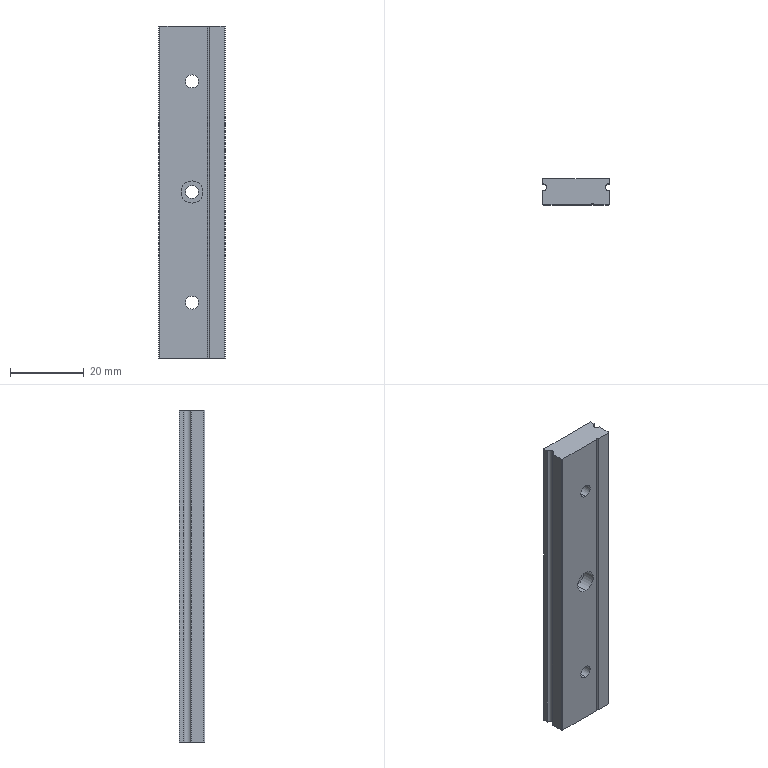Part | STEP file | Mount electronic clip MGW9H rail | 1 solid | 30 faces | box 18 x 7 x 90 mm | volume 10639 mm3 | cylinder 16 | plane 14 | commonest cylinder face diameters 3.5 x6 6 x6 2 x3 0.6 x1